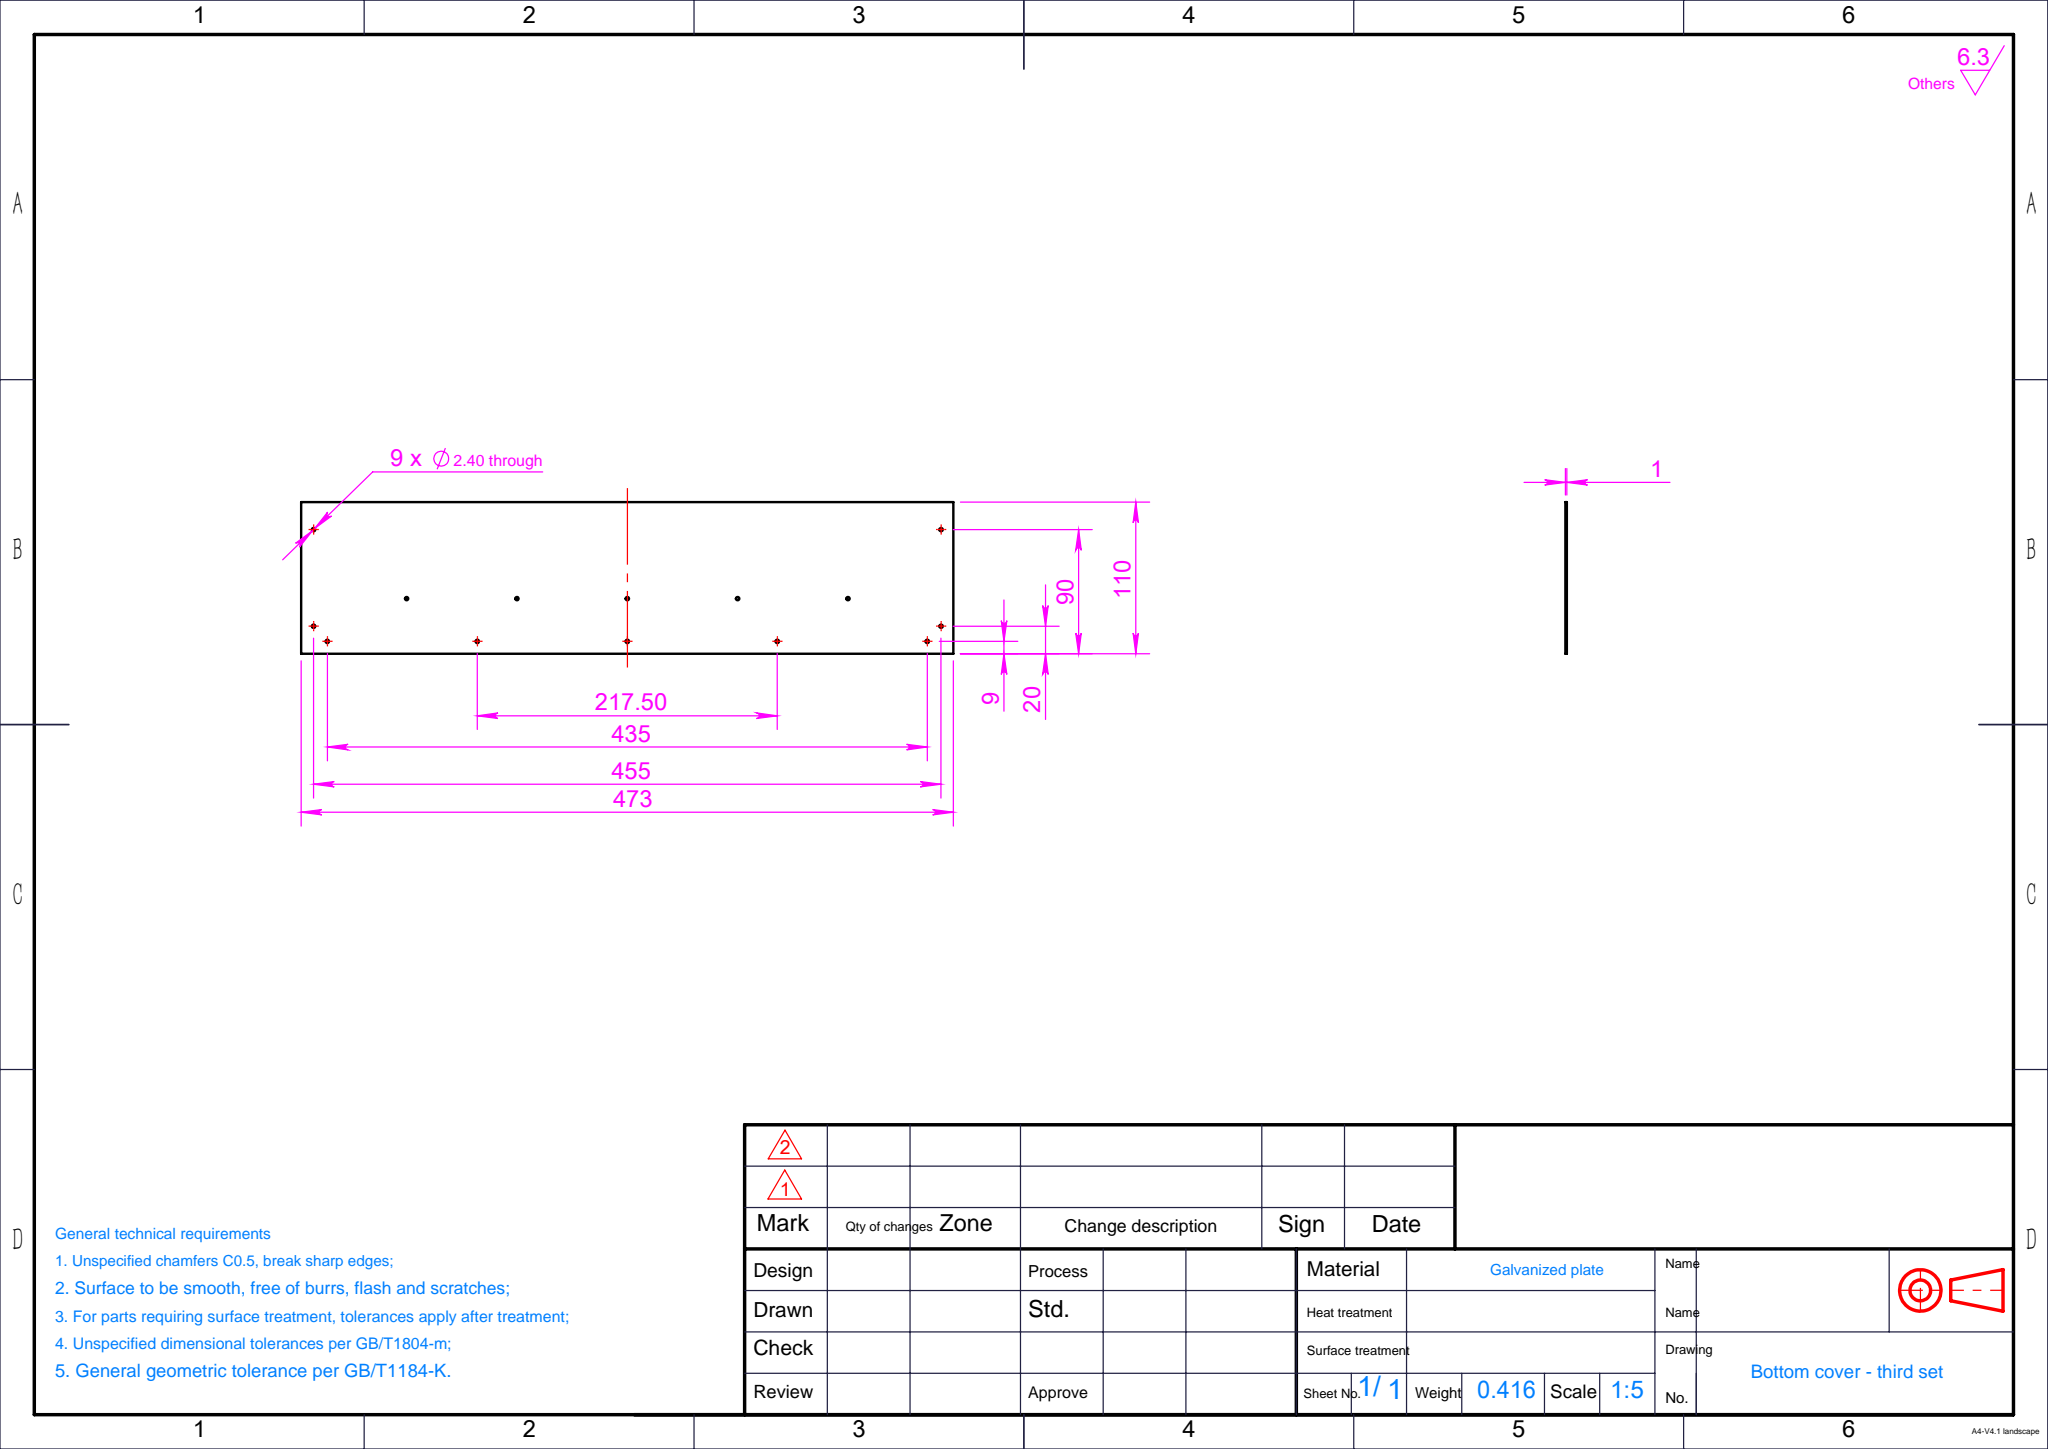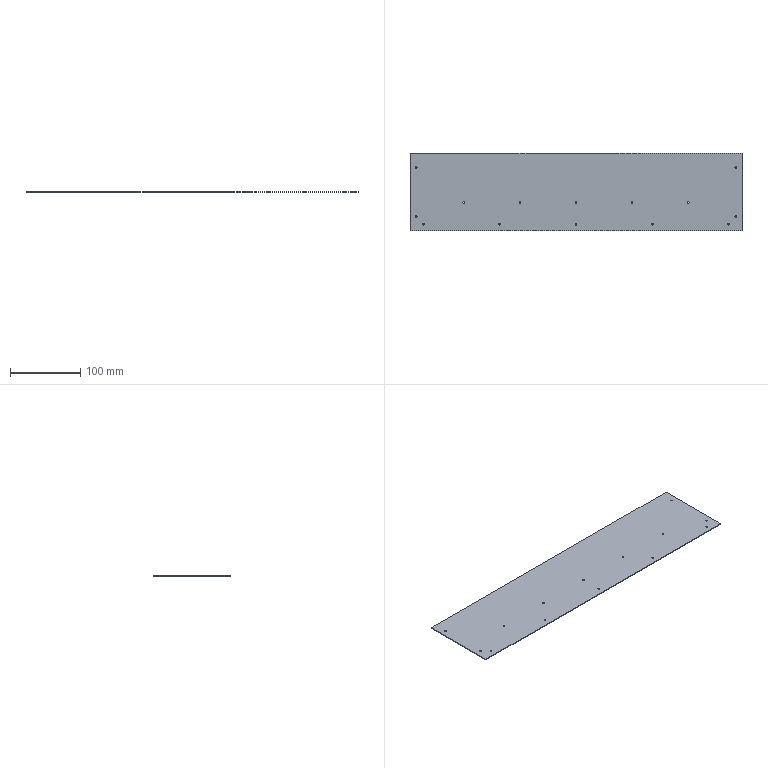Part | SolidWorks | features 3DProfileFeature 1, Chamfer 1, FlatPattern 1, HoleWzd 1, SMBaseFlange 1, SheetMetal 1, SketchPattern 1 | 1 solid | 34 faces | box 473 x 110 x 1 mm | volume 51967 mm3 | cylinder 28 | plane 6 | commonest cylinder face diameters 2.4 x28